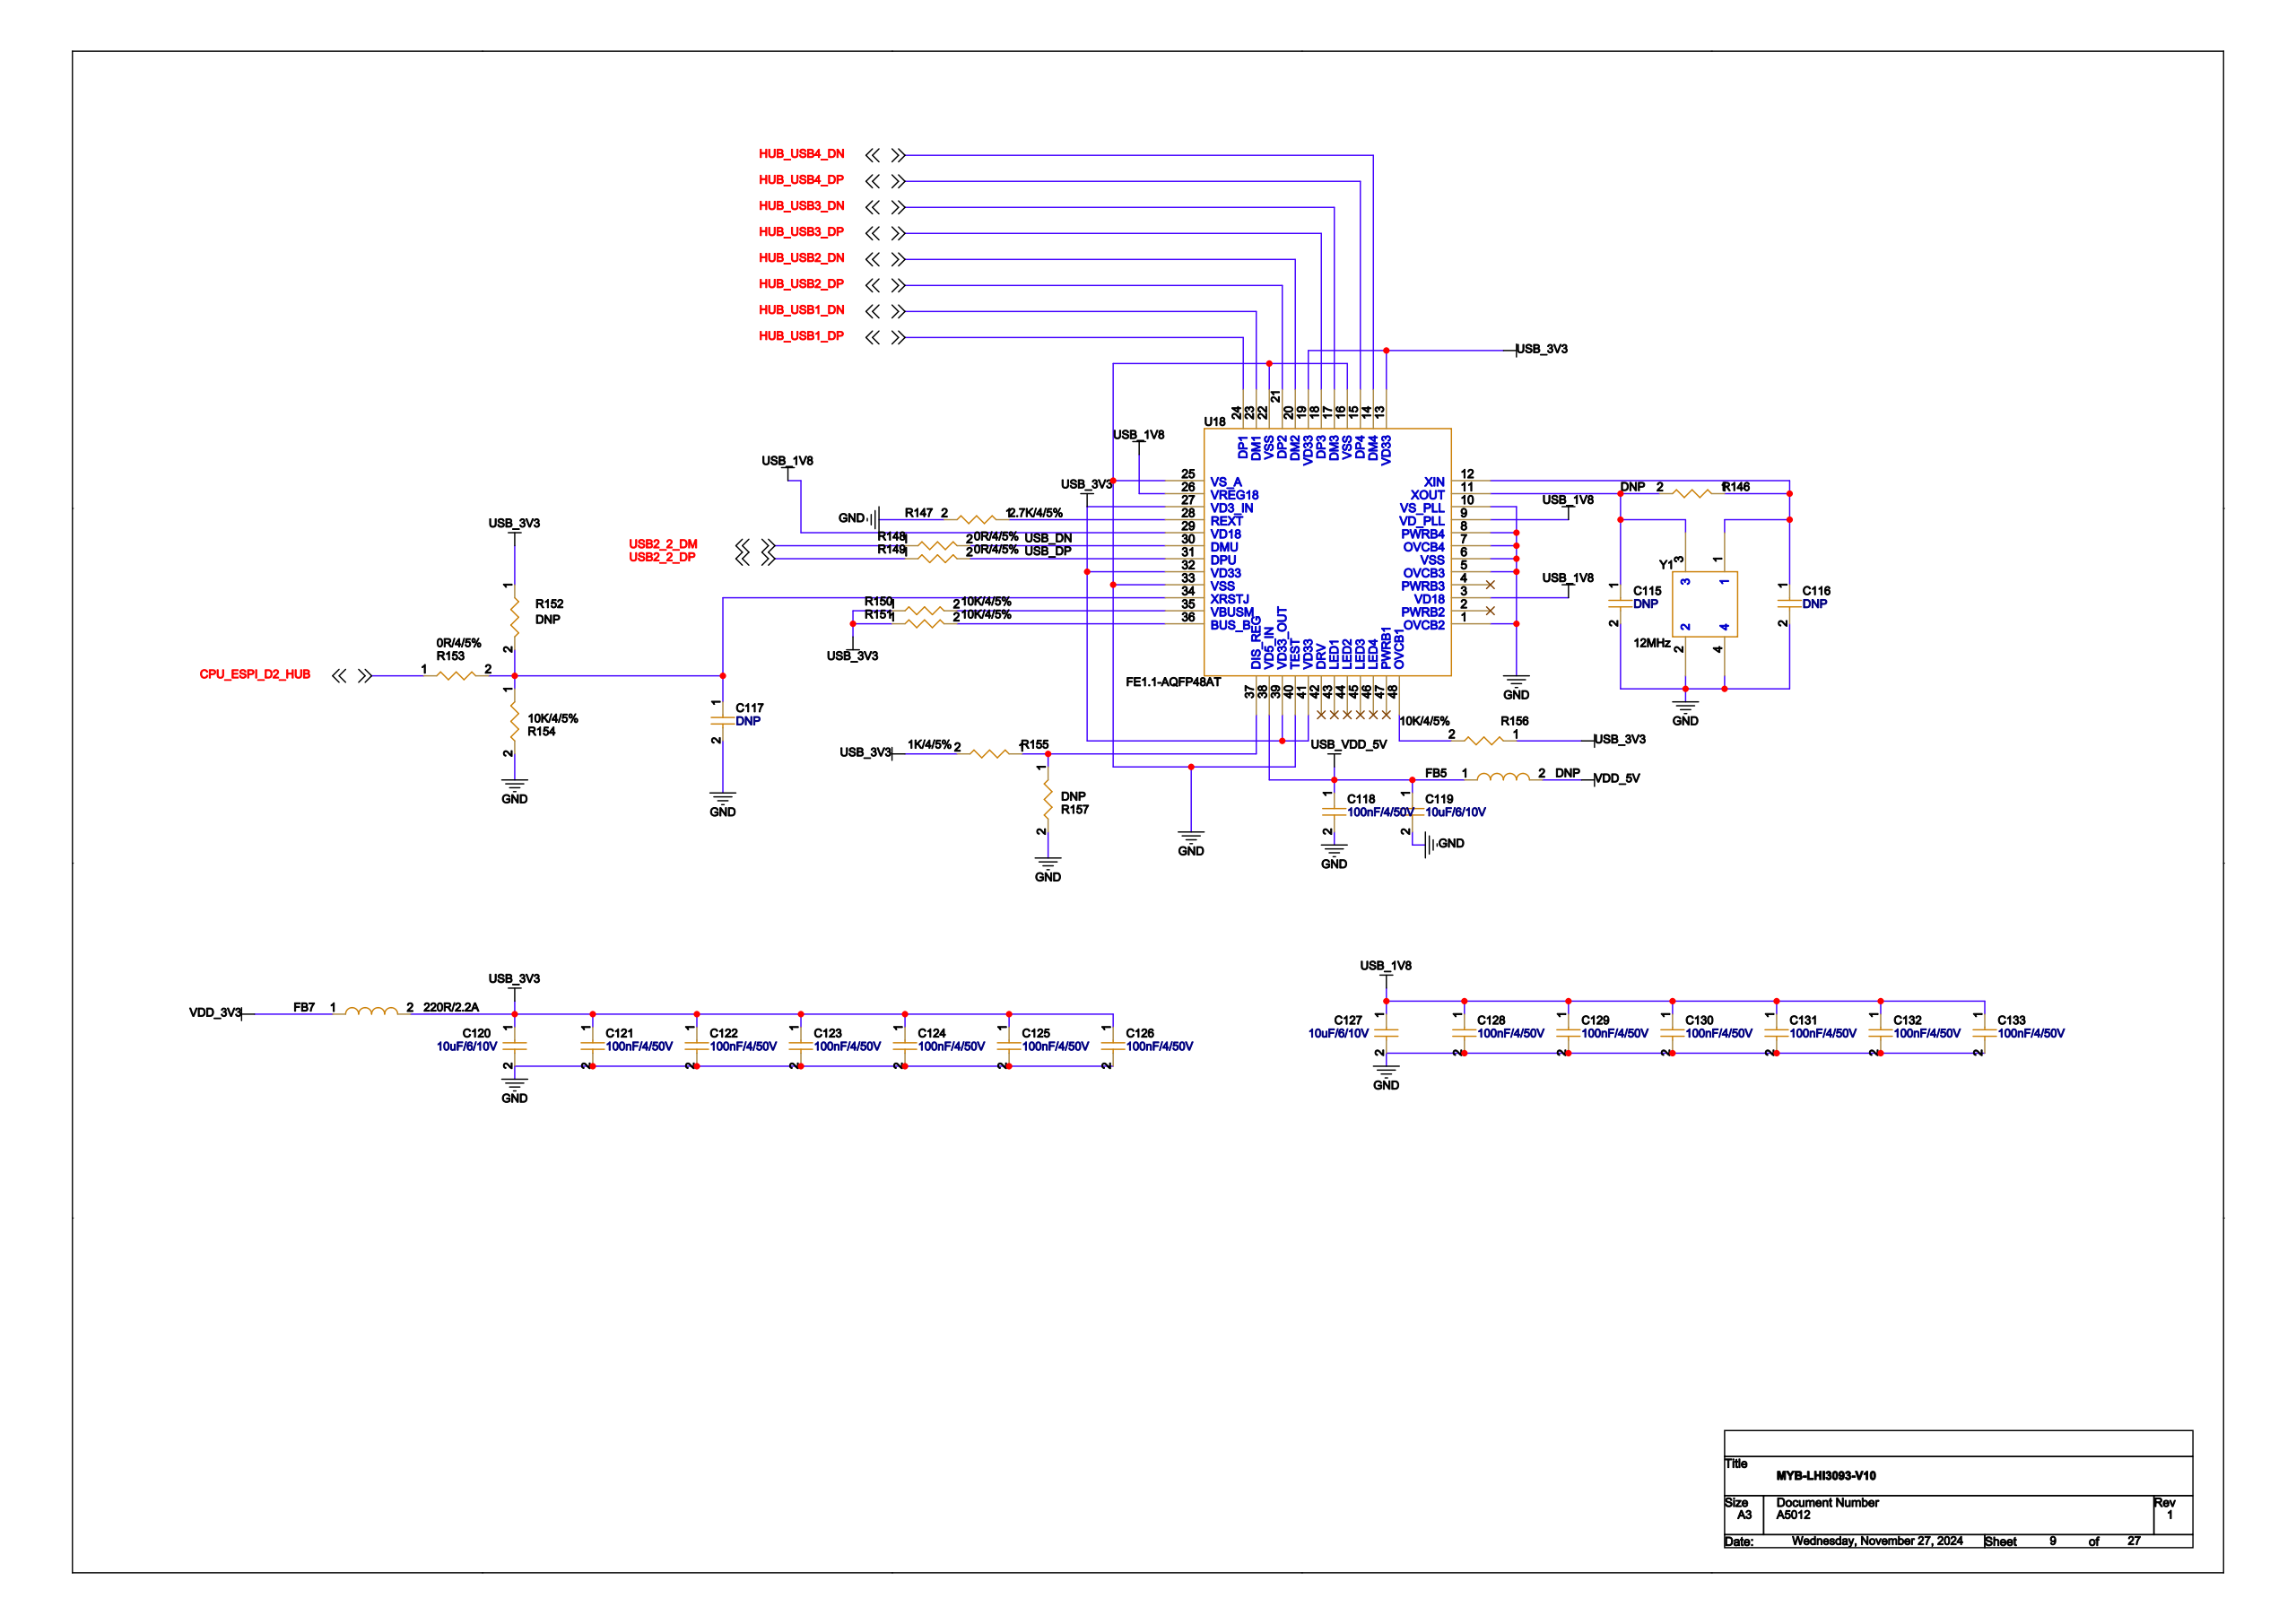Circuit board | Cadence Allegro | 1159 parts | 708 nets | one sheet of the schematic
Parts on this sheet (reference | value | footprint):
C115 | DNP | C0402
C116 | DNP | C0402
C117 | DNP | C0402
C118 | 100nF/4/50V | C0402
C119 | 10uF/6/10V | C0603
C120 | 10uF/6/10V | C0603
C121 | 100nF/4/50V | C0402
C122 | 100nF/4/50V | C0402
C123 | 100nF/4/50V | C0402
C124 | 100nF/4/50V | C0402
C125 | 100nF/4/50V | C0402
C126 | 100nF/4/50V | C0402
C127 | 10uF/6/10V | C0603
C128 | 100nF/4/50V | C0402
C129 | 100nF/4/50V | C0402
C130 | 100nF/4/50V | C0402
C131 | 100nF/4/50V | C0402
C132 | 100nF/4/50V | C0402
C133 | 100nF/4/50V | C0402
FB5 | DNP | FB0603
FB7 | 220R/2.2A | FB0603
R147 | 2.7K/4/5% | R0402
R152 | DNP | R0402
R153 | 0R/4/5% | R0402
R154 | 10K/4/5% | R0402
R156 | 10K/4/5% | R0402
R157 | DNP | R0402
U18 | FE1.1-AQFP48AT | LQFP48
Y1 | 12MHz | 3225
Nets of these parts (net: part-pin ...):
GND: C115-2 C116-2 C117-2 C118-2 C119-2 C120-2 C121-2 C122-2 C123-2 C124-2 C125-2 C126-2 C127-2 C128-2 C129-2 C130-2 C131-2 C132-2 C133-2 R147-2 R154-2 R157-2 Y1-2 Y1-4 U18-1 U18-5 U18-6 U18-7 U18-8 U18-10 U18-16 U18-22 U18-25 U18-33 U18-40
VDD_5V: FB5-2
VDD_3V3: FB7-1
USB_VDD_5V: C118-1 C119-1 FB5-1 U18-38
USB_3V3: C120-1 C121-1 C122-1 C123-1 C124-1 C125-1 C126-1 FB7-2 R152-1 R156-1 U18-13 U18-19 U18-27 U18-32 U18-39 U18-41
USB_1V8: C127-1 C128-1 C129-1 C130-1 C131-1 C132-1 C133-1 U18-3 U18-9 U18-26 U18-29
N14864276: C115-1 Y1-3 U18-11
N14864444: C116-1 Y1-1 U18-12
N14866980: C117-1 R152-2 R153-2 R154-1 U18-34
HUB_USB1_DN: U18-23
HUB_USB1_DP: U18-24
HUB_USB4_DN: U18-14
HUB_USB4_DP: U18-15
HUB_USB2_DP: U18-21
HUB_USB2_DN: U18-20
USB_DN: U18-30
USB_DP: U18-31
CPU_ESPI_D2_HUB: R153-1
N14865297: R156-2 U18-48
N14866113: R157-1 U18-37
N15177061: R147-1 U18-28
HUB_USB3_DN: U18-17
HUB_USB3_DP: U18-18